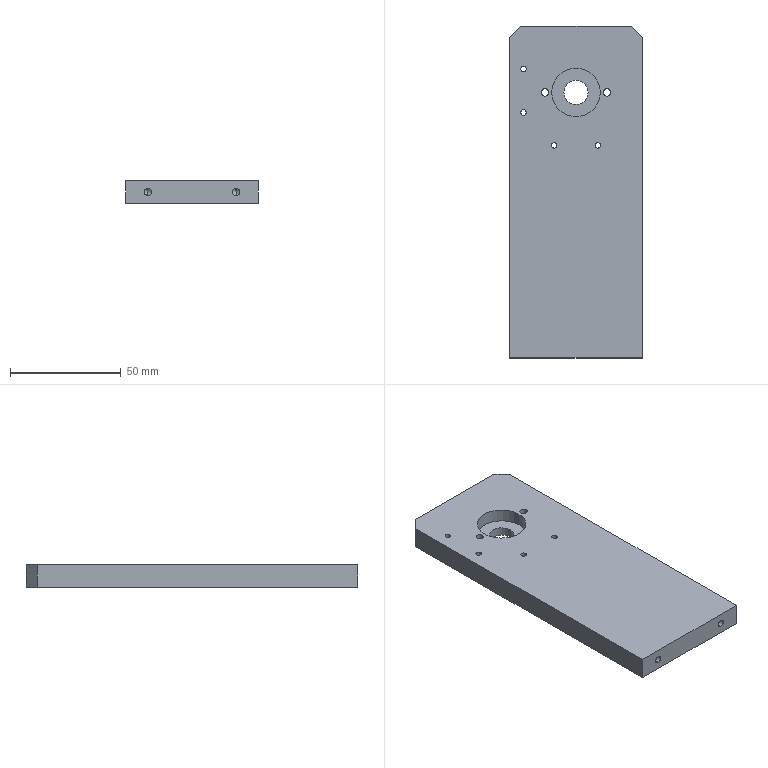Part | SolidWorks | features HoleWzd 3, ICE 2, Chamfer 1, Extrusion 1 | 1 solid | 33 faces | box 60 x 150 x 10 mm | volume 86519 mm3 | cylinder 20 | plane 9 | cone 4 | commonest cylinder face diameters 2.5 x8 3.3 x8 11 x2 22 x2
STEP:
#1=CARTESIAN_POINT('',(11.1,21.1,10.));
#2=VERTEX_POINT('',#1);
#3=CARTESIAN_POINT('',(8.6,21.1,10.));
#4=VERTEX_POINT('',#3);
#5=CARTESIAN_POINT('',(9.85,21.1,10.));
#6=DIRECTION('',(0.,0.,-1.));
#7=DIRECTION('',(-1.,0.,0.));
#8=AXIS2_PLACEMENT_3D('',#5,#6,#7);
#9=CIRCLE('',#8,1.25);
#10=EDGE_CURVE('',#2,#4,#9,.T.);
#11=ORIENTED_EDGE('',*,*,#10,.F.);
#12=CARTESIAN_POINT('',(11.1,21.1,0.));
#13=VERTEX_POINT('',#12);
#14=CARTESIAN_POINT('',(11.1,21.1,0.));
#15=DIRECTION('',(0.,0.,-1.));
#16=VECTOR('',#15,1000.);
#17=LINE('',#14,#16);
#18=EDGE_CURVE('',#2,#13,#17,.T.);
#19=ORIENTED_EDGE('',*,*,#18,.T.);
#20=CARTESIAN_POINT('',(8.6,21.1,0.));
#21=VERTEX_POINT('',#20);
#22=CARTESIAN_POINT('',(9.85,21.1,0.));
#23=DIRECTION('',(0.,0.,-1.));
#24=DIRECTION('',(-1.,0.,0.));
#25=AXIS2_PLACEMENT_3D('',#22,#23,#24);
#26=CIRCLE('',#25,1.25);
#27=EDGE_CURVE('',#13,#21,#26,.T.);
#28=ORIENTED_EDGE('',*,*,#27,.T.);
#29=CARTESIAN_POINT('',(8.6,21.1,0.));
#30=DIRECTION('',(0.,0.,-1.));
#31=VECTOR('',#30,1000.);
#32=LINE('',#29,#31);
#33=EDGE_CURVE('',#4,#21,#32,.T.);
#34=ORIENTED_EDGE('',*,*,#33,.F.);
#35=EDGE_LOOP('',(#11,#19,#28,#34));
#36=FACE_OUTER_BOUND('',#35,.T.);
#37=CARTESIAN_POINT('',(9.85,21.1,0.));
#38=DIRECTION('',(0.,0.,-1.));
#39=DIRECTION('',(-1.,0.,0.));
#40=AXIS2_PLACEMENT_3D('',#37,#38,#39);
#41=CYLINDRICAL_SURFACE('',#40,1.25);
#42=ADVANCED_FACE('',(#36),#41,.F.);
#43=CARTESIAN_POINT('',(-8.6,21.1,10.));
#44=VERTEX_POINT('',#43);
#45=CARTESIAN_POINT('',(-11.1,21.1,10.));
#46=VERTEX_POINT('',#45);
#47=CARTESIAN_POINT('',(-9.85,21.1,10.));
#48=DIRECTION('',(0.,0.,-1.));
#49=DIRECTION('',(-1.,0.,0.));
#50=AXIS2_PLACEMENT_3D('',#47,#48,#49);
#51=CIRCLE('',#50,1.25);
#52=EDGE_CURVE('',#44,#46,#51,.T.);
#53=ORIENTED_EDGE('',*,*,#52,.F.);
#54=CARTESIAN_POINT('',(-8.6,21.1,0.));
#55=VERTEX_POINT('',#54);
#56=CARTESIAN_POINT('',(-8.6,21.1,0.));
#57=DIRECTION('',(0.,0.,-1.));
#58=VECTOR('',#57,1000.);
#59=LINE('',#56,#58);
#60=EDGE_CURVE('',#44,#55,#59,.T.);
#61=ORIENTED_EDGE('',*,*,#60,.T.);
#62=CARTESIAN_POINT('',(-11.1,21.1,0.));
#63=VERTEX_POINT('',#62);
#64=CARTESIAN_POINT('',(-9.85,21.1,0.));
#65=DIRECTION('',(0.,0.,-1.));
#66=DIRECTION('',(-1.,0.,0.));
#67=AXIS2_PLACEMENT_3D('',#64,#65,#66);
#68=CIRCLE('',#67,1.25);
#69=EDGE_CURVE('',#55,#63,#68,.T.);
#70=ORIENTED_EDGE('',*,*,#69,.T.);
#71=CARTESIAN_POINT('',(-11.1,21.1,0.));
#72=DIRECTION('',(0.,0.,-1.));
#73=VECTOR('',#72,1000.);
#74=LINE('',#71,#73);
#75=EDGE_CURVE('',#46,#63,#74,.T.);
#76=ORIENTED_EDGE('',*,*,#75,.F.);
#77=EDGE_LOOP('',(#53,#61,#70,#76));
#78=FACE_OUTER_BOUND('',#77,.T.);
#79=CARTESIAN_POINT('',(-9.85,21.1,0.));
#80=DIRECTION('',(0.,0.,-1.));
#81=DIRECTION('',(-1.,0.,0.));
#82=AXIS2_PLACEMENT_3D('',#79,#80,#81);
#83=CYLINDRICAL_SURFACE('',#82,1.25);
#84=ADVANCED_FACE('',(#78),#83,.F.);
#85=CARTESIAN_POINT('',(-22.45,35.95,10.));
#86=VERTEX_POINT('',#85);
#87=CARTESIAN_POINT('',(-24.95,35.95,10.));
#88=VERTEX_POINT('',#87);
#89=CARTESIAN_POINT('',(-23.7,35.95,10.));
#90=DIRECTION('',(0.,0.,-1.));
#91=DIRECTION('',(-1.,0.,0.));
#92=AXIS2_PLACEMENT_3D('',#89,#90,#91);
#93=CIRCLE('',#92,1.25);
#94=EDGE_CURVE('',#86,#88,#93,.T.);
#95=ORIENTED_EDGE('',*,*,#94,.F.);
#96=CARTESIAN_POINT('',(-22.45,35.95,0.));
#97=VERTEX_POINT('',#96);
#98=CARTESIAN_POINT('',(-22.45,35.95,0.));
#99=DIRECTION('',(0.,0.,-1.));
#100=VECTOR('',#99,1000.);
#101=LINE('',#98,#100);
#102=EDGE_CURVE('',#86,#97,#101,.T.);
#103=ORIENTED_EDGE('',*,*,#102,.T.);
#104=CARTESIAN_POINT('',(-24.95,35.95,0.));
#105=VERTEX_POINT('',#104);
#106=CARTESIAN_POINT('',(-23.7,35.95,0.));
#107=DIRECTION('',(0.,0.,-1.));
#108=DIRECTION('',(-1.,0.,0.));
#109=AXIS2_PLACEMENT_3D('',#106,#107,#108);
#110=CIRCLE('',#109,1.25);
#111=EDGE_CURVE('',#97,#105,#110,.T.);
#112=ORIENTED_EDGE('',*,*,#111,.T.);
#113=CARTESIAN_POINT('',(-24.95,35.95,0.));
#114=DIRECTION('',(0.,0.,-1.));
#115=VECTOR('',#114,1000.);
#116=LINE('',#113,#115);
#117=EDGE_CURVE('',#88,#105,#116,.T.);
#118=ORIENTED_EDGE('',*,*,#117,.F.);
#119=EDGE_LOOP('',(#95,#103,#112,#118));
#120=FACE_OUTER_BOUND('',#119,.T.);
#121=CARTESIAN_POINT('',(-23.7,35.95,0.));
#122=DIRECTION('',(0.,0.,-1.));
#123=DIRECTION('',(-1.,0.,0.));
#124=AXIS2_PLACEMENT_3D('',#121,#122,#123);
#125=CYLINDRICAL_SURFACE('',#124,1.25);
#126=ADVANCED_FACE('',(#120),#125,.F.);
#127=CARTESIAN_POINT('',(-22.45,55.65,10.));
#128=VERTEX_POINT('',#127);
#129=CARTESIAN_POINT('',(-24.95,55.65,10.));
#130=VERTEX_POINT('',#129);
#131=CARTESIAN_POINT('',(-23.7,55.65,10.));
#132=DIRECTION('',(0.,0.,-1.));
#133=DIRECTION('',(-1.,0.,0.));
#134=AXIS2_PLACEMENT_3D('',#131,#132,#133);
#135=CIRCLE('',#134,1.25);
#136=EDGE_CURVE('',#128,#130,#135,.T.);
#137=ORIENTED_EDGE('',*,*,#136,.F.);
#138=CARTESIAN_POINT('',(-22.45,55.65,0.));
#139=VERTEX_POINT('',#138);
#140=CARTESIAN_POINT('',(-22.45,55.65,0.));
#141=DIRECTION('',(0.,0.,-1.));
#142=VECTOR('',#141,1000.);
#143=LINE('',#140,#142);
#144=EDGE_CURVE('',#128,#139,#143,.T.);
#145=ORIENTED_EDGE('',*,*,#144,.T.);
#146=CARTESIAN_POINT('',(-24.95,55.65,0.));
#147=VERTEX_POINT('',#146);
#148=CARTESIAN_POINT('',(-23.7,55.65,0.));
#149=DIRECTION('',(0.,0.,-1.));
#150=DIRECTION('',(-1.,0.,0.));
#151=AXIS2_PLACEMENT_3D('',#148,#149,#150);
#152=CIRCLE('',#151,1.25);
#153=EDGE_CURVE('',#139,#147,#152,.T.);
#154=ORIENTED_EDGE('',*,*,#153,.T.);
#155=CARTESIAN_POINT('',(-24.95,55.65,0.));
#156=DIRECTION('',(0.,0.,-1.));
#157=VECTOR('',#156,1000.);
#158=LINE('',#155,#157);
#159=EDGE_CURVE('',#130,#147,#158,.T.);
#160=ORIENTED_EDGE('',*,*,#159,.F.);
#161=EDGE_LOOP('',(#137,#145,#154,#160));
#162=FACE_OUTER_BOUND('',#161,.T.);
#163=CARTESIAN_POINT('',(-23.7,55.65,0.));
#164=DIRECTION('',(0.,0.,-1.));
#165=DIRECTION('',(-1.,0.,0.));
#166=AXIS2_PLACEMENT_3D('',#163,#164,#165);
#167=CYLINDRICAL_SURFACE('',#166,1.25);
#168=ADVANCED_FACE('',(#162),#167,.F.);
#169=CARTESIAN_POINT('',(20.,-63.5,6.65));
#170=VERTEX_POINT('',#169);
#171=CARTESIAN_POINT('',(20.,-63.5,3.35));
#172=VERTEX_POINT('',#171);
#173=CARTESIAN_POINT('',(20.,-63.5,5.));
#174=DIRECTION('',(0.,-1.,0.));
#175=DIRECTION('',(0.,0.,-1.));
#176=AXIS2_PLACEMENT_3D('',#173,#174,#175);
#177=CIRCLE('',#176,1.65);
#178=EDGE_CURVE('',#170,#172,#177,.T.);
#179=ORIENTED_EDGE('',*,*,#178,.F.);
#180=CARTESIAN_POINT('',(20.,-75.,6.65));
#181=VERTEX_POINT('',#180);
#182=CARTESIAN_POINT('',(20.,-75.,6.65));
#183=DIRECTION('',(0.,-1.,0.));
#184=VECTOR('',#183,1000.);
#185=LINE('',#182,#184);
#186=EDGE_CURVE('',#170,#181,#185,.T.);
#187=ORIENTED_EDGE('',*,*,#186,.T.);
#188=CARTESIAN_POINT('',(20.,-75.,3.35));
#189=VERTEX_POINT('',#188);
#190=CARTESIAN_POINT('',(20.,-75.,5.));
#191=DIRECTION('',(0.,-1.,0.));
#192=DIRECTION('',(0.,0.,-1.));
#193=AXIS2_PLACEMENT_3D('',#190,#191,#192);
#194=CIRCLE('',#193,1.65);
#195=EDGE_CURVE('',#181,#189,#194,.T.);
#196=ORIENTED_EDGE('',*,*,#195,.T.);
#197=CARTESIAN_POINT('',(20.,-75.,3.35));
#198=DIRECTION('',(0.,-1.,0.));
#199=VECTOR('',#198,1000.);
#200=LINE('',#197,#199);
#201=EDGE_CURVE('',#172,#189,#200,.T.);
#202=ORIENTED_EDGE('',*,*,#201,.F.);
#203=EDGE_LOOP('',(#179,#187,#196,#202));
#204=FACE_OUTER_BOUND('',#203,.T.);
#205=CARTESIAN_POINT('',(20.,-75.,5.));
#206=DIRECTION('',(0.,-1.,0.));
#207=DIRECTION('',(0.,0.,-1.));
#208=AXIS2_PLACEMENT_3D('',#205,#206,#207);
#209=CYLINDRICAL_SURFACE('',#208,1.65);
#210=ADVANCED_FACE('',(#204),#209,.F.);
#211=CARTESIAN_POINT('',(20.,-62.509,5.));
#212=VERTEX_POINT('',#211);
#213=CARTESIAN_POINT('',(20.,-63.5,3.35));
#214=DIRECTION('',(0.,-0.515,-0.8572));
#215=VECTOR('',#214,1000.);
#216=LINE('',#213,#215);
#217=EDGE_CURVE('',#212,#172,#216,.T.);
#218=ORIENTED_EDGE('',*,*,#217,.F.);
#219=CARTESIAN_POINT('',(20.,-63.5,6.65));
#220=DIRECTION('',(0.,-0.515,0.8572));
#221=VECTOR('',#220,1000.);
#222=LINE('',#219,#221);
#223=EDGE_CURVE('',#212,#170,#222,.T.);
#224=ORIENTED_EDGE('',*,*,#223,.T.);
#225=ORIENTED_EDGE('',*,*,#178,.T.);
#226=EDGE_LOOP('',(#218,#224,#225));
#227=FACE_OUTER_BOUND('',#226,.T.);
#228=CARTESIAN_POINT('',(20.,-63.5,5.));
#229=DIRECTION('',(0.,-1.,0.));
#230=DIRECTION('',(0.,0.,-1.));
#231=AXIS2_PLACEMENT_3D('',#228,#229,#230);
#232=CONICAL_SURFACE('',#231,1.65,1.03);
#233=ADVANCED_FACE('',(#227),#232,.F.);
#234=CARTESIAN_POINT('',(-20.,-63.5,6.65));
#235=VERTEX_POINT('',#234);
#236=CARTESIAN_POINT('',(-20.,-63.5,3.35));
#237=VERTEX_POINT('',#236);
#238=CARTESIAN_POINT('',(-20.,-63.5,5.));
#239=DIRECTION('',(0.,-1.,0.));
#240=DIRECTION('',(0.,0.,-1.));
#241=AXIS2_PLACEMENT_3D('',#238,#239,#240);
#242=CIRCLE('',#241,1.65);
#243=EDGE_CURVE('',#235,#237,#242,.T.);
#244=ORIENTED_EDGE('',*,*,#243,.F.);
#245=CARTESIAN_POINT('',(-20.,-75.,6.65));
#246=VERTEX_POINT('',#245);
#247=CARTESIAN_POINT('',(-20.,-75.,6.65));
#248=DIRECTION('',(0.,-1.,0.));
#249=VECTOR('',#248,1000.);
#250=LINE('',#247,#249);
#251=EDGE_CURVE('',#235,#246,#250,.T.);
#252=ORIENTED_EDGE('',*,*,#251,.T.);
#253=CARTESIAN_POINT('',(-20.,-75.,3.35));
#254=VERTEX_POINT('',#253);
#255=CARTESIAN_POINT('',(-20.,-75.,5.));
#256=DIRECTION('',(0.,-1.,0.));
#257=DIRECTION('',(0.,0.,-1.));
#258=AXIS2_PLACEMENT_3D('',#255,#256,#257);
#259=CIRCLE('',#258,1.65);
#260=EDGE_CURVE('',#246,#254,#259,.T.);
#261=ORIENTED_EDGE('',*,*,#260,.T.);
#262=CARTESIAN_POINT('',(-20.,-75.,3.35));
#263=DIRECTION('',(0.,-1.,0.));
#264=VECTOR('',#263,1000.);
#265=LINE('',#262,#264);
#266=EDGE_CURVE('',#237,#254,#265,.T.);
#267=ORIENTED_EDGE('',*,*,#266,.F.);
#268=EDGE_LOOP('',(#244,#252,#261,#267));
#269=FACE_OUTER_BOUND('',#268,.T.);
#270=CARTESIAN_POINT('',(-20.,-75.,5.));
#271=DIRECTION('',(0.,-1.,0.));
#272=DIRECTION('',(0.,0.,-1.));
#273=AXIS2_PLACEMENT_3D('',#270,#271,#272);
#274=CYLINDRICAL_SURFACE('',#273,1.65);
#275=ADVANCED_FACE('',(#269),#274,.F.);
#276=CARTESIAN_POINT('',(-20.,-62.509,5.));
#277=VERTEX_POINT('',#276);
#278=CARTESIAN_POINT('',(-20.,-63.5,3.35));
#279=DIRECTION('',(0.,-0.515,-0.8572));
#280=VECTOR('',#279,1000.);
#281=LINE('',#278,#280);
#282=EDGE_CURVE('',#277,#237,#281,.T.);
#283=ORIENTED_EDGE('',*,*,#282,.F.);
#284=CARTESIAN_POINT('',(-20.,-63.5,6.65));
#285=DIRECTION('',(0.,-0.515,0.8572));
#286=VECTOR('',#285,1000.);
#287=LINE('',#284,#286);
#288=EDGE_CURVE('',#277,#235,#287,.T.);
#289=ORIENTED_EDGE('',*,*,#288,.T.);
#290=ORIENTED_EDGE('',*,*,#243,.T.);
#291=EDGE_LOOP('',(#283,#289,#290));
#292=FACE_OUTER_BOUND('',#291,.T.);
#293=CARTESIAN_POINT('',(-20.,-63.5,5.));
#294=DIRECTION('',(0.,-1.,0.));
#295=DIRECTION('',(0.,0.,-1.));
#296=AXIS2_PLACEMENT_3D('',#293,#294,#295);
#297=CONICAL_SURFACE('',#296,1.65,1.03);
#298=ADVANCED_FACE('',(#292),#297,.F.);
#299=CARTESIAN_POINT('',(-15.65,45.,0.));
#300=VERTEX_POINT('',#299);
#301=CARTESIAN_POINT('',(-12.35,45.,0.));
#302=VERTEX_POINT('',#301);
#303=CARTESIAN_POINT('',(-14.,45.,0.));
#304=DIRECTION('',(0.,0.,1.));
#305=DIRECTION('',(1.,0.,0.));
#306=AXIS2_PLACEMENT_3D('',#303,#304,#305);
#307=CIRCLE('',#306,1.65);
#308=EDGE_CURVE('',#300,#302,#307,.T.);
#309=ORIENTED_EDGE('',*,*,#308,.F.);
#310=CARTESIAN_POINT('',(-15.65,45.,10.));
#311=VERTEX_POINT('',#310);
#312=CARTESIAN_POINT('',(-15.65,45.,10.));
#313=DIRECTION('',(0.,0.,1.));
#314=VECTOR('',#313,1000.);
#315=LINE('',#312,#314);
#316=EDGE_CURVE('',#300,#311,#315,.T.);
#317=ORIENTED_EDGE('',*,*,#316,.T.);
#318=CARTESIAN_POINT('',(-12.35,45.,10.));
#319=VERTEX_POINT('',#318);
#320=CARTESIAN_POINT('',(-14.,45.,10.));
#321=DIRECTION('',(0.,0.,1.));
#322=DIRECTION('',(1.,0.,0.));
#323=AXIS2_PLACEMENT_3D('',#320,#321,#322);
#324=CIRCLE('',#323,1.65);
#325=EDGE_CURVE('',#311,#319,#324,.T.);
#326=ORIENTED_EDGE('',*,*,#325,.T.);
#327=CARTESIAN_POINT('',(-12.35,45.,10.));
#328=DIRECTION('',(0.,0.,1.));
#329=VECTOR('',#328,1000.);
#330=LINE('',#327,#329);
#331=EDGE_CURVE('',#302,#319,#330,.T.);
#332=ORIENTED_EDGE('',*,*,#331,.F.);
#333=EDGE_LOOP('',(#309,#317,#326,#332));
#334=FACE_OUTER_BOUND('',#333,.T.);
#335=CARTESIAN_POINT('',(-14.,45.,10.));
#336=DIRECTION('',(0.,0.,1.));
#337=DIRECTION('',(1.,0.,0.));
#338=AXIS2_PLACEMENT_3D('',#335,#336,#337);
#339=CYLINDRICAL_SURFACE('',#338,1.65);
#340=ADVANCED_FACE('',(#334),#339,.F.);
#341=CARTESIAN_POINT('',(12.35,45.,0.));
#342=VERTEX_POINT('',#341);
#343=CARTESIAN_POINT('',(15.65,45.,0.));
#344=VERTEX_POINT('',#343);
#345=CARTESIAN_POINT('',(14.,45.,0.));
#346=DIRECTION('',(0.,0.,1.));
#347=DIRECTION('',(1.,0.,0.));
#348=AXIS2_PLACEMENT_3D('',#345,#346,#347);
#349=CIRCLE('',#348,1.65);
#350=EDGE_CURVE('',#342,#344,#349,.T.);
#351=ORIENTED_EDGE('',*,*,#350,.F.);
#352=CARTESIAN_POINT('',(12.35,45.,10.));
#353=VERTEX_POINT('',#352);
#354=CARTESIAN_POINT('',(12.35,45.,10.));
#355=DIRECTION('',(0.,0.,1.));
#356=VECTOR('',#355,1000.);
#357=LINE('',#354,#356);
#358=EDGE_CURVE('',#342,#353,#357,.T.);
#359=ORIENTED_EDGE('',*,*,#358,.T.);
#360=CARTESIAN_POINT('',(15.65,45.,10.));
#361=VERTEX_POINT('',#360);
#362=CARTESIAN_POINT('',(14.,45.,10.));
#363=DIRECTION('',(0.,0.,1.));
#364=DIRECTION('',(1.,0.,0.));
#365=AXIS2_PLACEMENT_3D('',#362,#363,#364);
#366=CIRCLE('',#365,1.65);
#367=EDGE_CURVE('',#353,#361,#366,.T.);
#368=ORIENTED_EDGE('',*,*,#367,.T.);
#369=CARTESIAN_POINT('',(15.65,45.,10.));
#370=DIRECTION('',(0.,0.,1.));
#371=VECTOR('',#370,1000.);
#372=LINE('',#369,#371);
#373=EDGE_CURVE('',#344,#361,#372,.T.);
#374=ORIENTED_EDGE('',*,*,#373,.F.);
#375=EDGE_LOOP('',(#351,#359,#368,#374));
#376=FACE_OUTER_BOUND('',#375,.T.);
#377=CARTESIAN_POINT('',(14.,45.,10.));
#378=DIRECTION('',(0.,0.,1.));
#379=DIRECTION('',(1.,0.,0.));
#380=AXIS2_PLACEMENT_3D('',#377,#378,#379);
#381=CYLINDRICAL_SURFACE('',#380,1.65);
#382=ADVANCED_FACE('',(#376),#381,.F.);
#383=CARTESIAN_POINT('',(-5.5,45.,0.));
#384=VERTEX_POINT('',#383);
#385=CARTESIAN_POINT('',(5.5,45.,0.));
#386=VERTEX_POINT('',#385);
#387=CARTESIAN_POINT('',(0.,45.,0.));
#388=DIRECTION('',(0.,0.,1.));
#389=DIRECTION('',(1.,0.,0.));
#390=AXIS2_PLACEMENT_3D('',#387,#388,#389);
#391=CIRCLE('',#390,5.5);
#392=EDGE_CURVE('',#384,#386,#391,.T.);
#393=ORIENTED_EDGE('',*,*,#392,.F.);
#394=CARTESIAN_POINT('',(-5.5,45.,4.));
#395=VERTEX_POINT('',#394);
#396=CARTESIAN_POINT('',(-5.5,45.,0.));
#397=DIRECTION('',(0.,0.,1.));
#398=VECTOR('',#397,1000.);
#399=LINE('',#396,#398);
#400=EDGE_CURVE('',#384,#395,#399,.T.);
#401=ORIENTED_EDGE('',*,*,#400,.T.);
#402=CARTESIAN_POINT('',(5.5,45.,4.));
#403=VERTEX_POINT('',#402);
#404=CARTESIAN_POINT('',(0.,45.,4.));
#405=DIRECTION('',(0.,0.,1.));
#406=DIRECTION('',(1.,0.,0.));
#407=AXIS2_PLACEMENT_3D('',#404,#405,#406);
#408=CIRCLE('',#407,5.5);
#409=EDGE_CURVE('',#395,#403,#408,.T.);
#410=ORIENTED_EDGE('',*,*,#409,.T.);
#411=CARTESIAN_POINT('',(5.5,45.,0.));
#412=DIRECTION('',(0.,0.,1.));
#413=VECTOR('',#412,1000.);
#414=LINE('',#411,#413);
#415=EDGE_CURVE('',#386,#403,#414,.T.);
#416=ORIENTED_EDGE('',*,*,#415,.F.);
#417=EDGE_LOOP('',(#393,#401,#410,#416));
#418=FACE_OUTER_BOUND('',#417,.T.);
#419=CARTESIAN_POINT('',(0.,45.,0.));
#420=DIRECTION('',(0.,0.,1.));
#421=DIRECTION('',(1.,0.,0.));
#422=AXIS2_PLACEMENT_3D('',#419,#420,#421);
#423=CYLINDRICAL_SURFACE('',#422,5.5);
#424=ADVANCED_FACE('',(#418),#423,.F.);
#425=CARTESIAN_POINT('',(-11.,45.,4.));
#426=VERTEX_POINT('',#425);
#427=CARTESIAN_POINT('',(11.,45.,4.));
#428=VERTEX_POINT('',#427);
#429=CARTESIAN_POINT('',(0.,45.,4.));
#430=DIRECTION('',(0.,0.,1.));
#431=DIRECTION('',(1.,0.,0.));
#432=AXIS2_PLACEMENT_3D('',#429,#430,#431);
#433=CIRCLE('',#432,11.);
#434=EDGE_CURVE('',#426,#428,#433,.T.);
#435=ORIENTED_EDGE('',*,*,#434,.F.);
#436=CARTESIAN_POINT('',(-11.,45.,10.));
#437=VERTEX_POINT('',#436);
#438=CARTESIAN_POINT('',(-11.,45.,4.));
#439=DIRECTION('',(0.,0.,1.));
#440=VECTOR('',#439,1000.);
#441=LINE('',#438,#440);
#442=EDGE_CURVE('',#426,#437,#441,.T.);
#443=ORIENTED_EDGE('',*,*,#442,.T.);
#444=CARTESIAN_POINT('',(11.,45.,10.));
#445=VERTEX_POINT('',#444);
#446=CARTESIAN_POINT('',(0.,45.,10.));
#447=DIRECTION('',(0.,0.,1.));
#448=DIRECTION('',(1.,0.,0.));
#449=AXIS2_PLACEMENT_3D('',#446,#447,#448);
#450=CIRCLE('',#449,11.);
#451=EDGE_CURVE('',#437,#445,#450,.T.);
#452=ORIENTED_EDGE('',*,*,#451,.T.);
#453=CARTESIAN_POINT('',(11.,45.,4.));
#454=DIRECTION('',(0.,0.,1.));
#455=VECTOR('',#454,1000.);
#456=LINE('',#453,#455);
#457=EDGE_CURVE('',#428,#445,#456,.T.);
#458=ORIENTED_EDGE('',*,*,#457,.F.);
#459=EDGE_LOOP('',(#435,#443,#452,#458));
#460=FACE_OUTER_BOUND('',#459,.T.);
#461=CARTESIAN_POINT('',(0.,45.,4.));
#462=DIRECTION('',(0.,0.,1.));
#463=DIRECTION('',(1.,0.,0.));
#464=AXIS2_PLACEMENT_3D('',#461,#462,#463);
#465=CYLINDRICAL_SURFACE('',#464,11.);
#466=ADVANCED_FACE('',(#460),#465,.F.);
#467=CARTESIAN_POINT('',(30.,-75.,0.));
#468=VERTEX_POINT('',#467);
#469=CARTESIAN_POINT('',(30.,70.,0.));
#470=VERTEX_POINT('',#469);
#471=CARTESIAN_POINT('',(30.,75.,0.));
#472=DIRECTION('',(0.,1.,0.));
#473=VECTOR('',#472,1000.);
#474=LINE('',#471,#473);
#475=EDGE_CURVE('',#468,#470,#474,.T.);
#476=ORIENTED_EDGE('',*,*,#475,.T.);
#477=CARTESIAN_POINT('',(30.,70.,10.));
#478=VERTEX_POINT('',#477);
#479=CARTESIAN_POINT('',(30.,70.,10.));
#480=DIRECTION('',(0.,0.,1.));
#481=VECTOR('',#480,1000.);
#482=LINE('',#479,#481);
#483=EDGE_CURVE('',#470,#478,#482,.T.);
#484=ORIENTED_EDGE('',*,*,#483,.T.);
#485=CARTESIAN_POINT('',(30.,-75.,10.));
#486=VERTEX_POINT('',#485);
#487=CARTESIAN_POINT('',(30.,75.,10.));
#488=DIRECTION('',(0.,1.,0.));
#489=VECTOR('',#488,1000.);
#490=LINE('',#487,#489);
#491=EDGE_CURVE('',#486,#478,#490,.T.);
#492=ORIENTED_EDGE('',*,*,#491,.F.);
#493=CARTESIAN_POINT('',(30.,-75.,10.));
#494=DIRECTION('',(0.,0.,-1.));
#495=VECTOR('',#494,1000.);
#496=LINE('',#493,#495);
#497=EDGE_CURVE('',#486,#468,#496,.T.);
#498=ORIENTED_EDGE('',*,*,#497,.T.);
#499=EDGE_LOOP('',(#476,#484,#492,#498));
#500=FACE_OUTER_BOUND('',#499,.T.);
#501=CARTESIAN_POINT('',(30.,75.,10.));
#502=DIRECTION('',(-1.,0.,0.));
#503=DIRECTION('',(0.,-1.,0.));
#504=AXIS2_PLACEMENT_3D('',#501,#502,#503);
#505=PLANE('',#504);
#506=ADVANCED_FACE('',(#500),#505,.F.);
#507=CARTESIAN_POINT('',(25.,75.,10.));
#508=VERTEX_POINT('',#507);
#509=CARTESIAN_POINT('',(-25.,75.,10.));
#510=VERTEX_POINT('',#509);
#511=CARTESIAN_POINT('',(-30.,75.,10.));
#512=DIRECTION('',(-1.,0.,0.));
#513=VECTOR('',#512,1000.);
#514=LINE('',#511,#513);
#515=EDGE_CURVE('',#508,#510,#514,.T.);
#516=ORIENTED_EDGE('',*,*,#515,.F.);
#517=CARTESIAN_POINT('',(25.,75.,0.));
#518=VERTEX_POINT('',#517);
#519=CARTESIAN_POINT('',(25.,75.,10.));
#520=DIRECTION('',(0.,0.,-1.));
#521=VECTOR('',#520,1000.);
#522=LINE('',#519,#521);
#523=EDGE_CURVE('',#508,#518,#522,.T.);
#524=ORIENTED_EDGE('',*,*,#523,.T.);
#525=CARTESIAN_POINT('',(-25.,75.,0.));
#526=VERTEX_POINT('',#525);
#527=CARTESIAN_POINT('',(-30.,75.,0.));
#528=DIRECTION('',(-1.,0.,0.));
#529=VECTOR('',#528,1000.);
#530=LINE('',#527,#529);
#531=EDGE_CURVE('',#518,#526,#530,.T.);
#532=ORIENTED_EDGE('',*,*,#531,.T.);
#533=CARTESIAN_POINT('',(-25.,75.,10.));
#534=DIRECTION('',(0.,0.,1.));
#535=VECTOR('',#534,1000.);
#536=LINE('',#533,#535);
#537=EDGE_CURVE('',#526,#510,#536,.T.);
#538=ORIENTED_EDGE('',*,*,#537,.T.);
#539=EDGE_LOOP('',(#516,#524,#532,#538));
#540=FACE_OUTER_BOUND('',#539,.T.);
#541=CARTESIAN_POINT('',(-30.,75.,10.));
#542=DIRECTION('',(0.,-1.,0.));
#543=DIRECTION('',(0.,0.,-1.));
#544=AXIS2_PLACEMENT_3D('',#541,#542,#543);
#545=PLANE('',#544);
#546=ADVANCED_FACE('',(#540),#545,.F.);
#547=CARTESIAN_POINT('',(-30.,70.,10.));
#548=VERTEX_POINT('',#547);
#549=CARTESIAN_POINT('',(-30.,-75.,10.));
#550=VERTEX_POINT('',#549);
#551=CARTESIAN_POINT('',(-30.,75.,10.));
#552=DIRECTION('',(0.,-1.,0.));
#553=VECTOR('',#552,1000.);
#554=LINE('',#551,#553);
#555=EDGE_CURVE('',#548,#550,#554,.T.);
#556=ORIENTED_EDGE('',*,*,#555,.F.);
#557=CARTESIAN_POINT('',(-30.,70.,0.));
#558=VERTEX_POINT('',#557);
#559=CARTESIAN_POINT('',(-30.,70.,10.));
#560=DIRECTION('',(0.,0.,-1.));
#561=VECTOR('',#560,1000.);
#562=LINE('',#559,#561);
#563=EDGE_CURVE('',#548,#558,#562,.T.);
#564=ORIENTED_EDGE('',*,*,#563,.T.);
#565=CARTESIAN_POINT('',(-30.,-75.,0.));
#566=VERTEX_POINT('',#565);
#567=CARTESIAN_POINT('',(-30.,75.,0.));
#568=DIRECTION('',(0.,-1.,0.));
#569=VECTOR('',#568,1000.);
#570=LINE('',#567,#569);
#571=EDGE_CURVE('',#558,#566,#570,.T.);
#572=ORIENTED_EDGE('',*,*,#571,.T.);
#573=CARTESIAN_POINT('',(-30.,-75.,10.));
#574=DIRECTION('',(0.,0.,-1.));
#575=VECTOR('',#574,1000.);
#576=LINE('',#573,#575);
#577=EDGE_CURVE('',#550,#566,#576,.T.);
#578=ORIENTED_EDGE('',*,*,#577,.F.);
#579=EDGE_LOOP('',(#556,#564,#572,#578));
#580=FACE_OUTER_BOUND('',#579,.T.);
#581=CARTESIAN_POINT('',(-30.,75.,10.));
#582=DIRECTION('',(1.,0.,0.));
#583=DIRECTION('',(0.,1.,0.));
#584=AXIS2_PLACEMENT_3D('',#581,#582,#583);
#585=PLANE('',#584);
#586=ADVANCED_FACE('',(#580),#585,.F.);
#587=CARTESIAN_POINT('',(20.,-75.,5.));
#588=DIRECTION('',(0.,-1.,0.));
#589=DIRECTION('',(0.,0.,-1.));
#590=AXIS2_PLACEMENT_3D('',#587,#588,#589);
#591=CIRCLE('',#590,1.65);
#592=EDGE_CURVE('',#189,#181,#591,.T.);
#593=ORIENTED_EDGE('',*,*,#592,.F.);
#594=ORIENTED_EDGE('',*,*,#195,.F.);
#595=EDGE_LOOP('',(#593,#594));
#596=FACE_BOUND('',#595,.T.);
#597=CARTESIAN_POINT('',(-20.,-75.,5.));
#598=DIRECTION('',(0.,-1.,0.));
#599=DIRECTION('',(0.,0.,-1.));
#600=AXIS2_PLACEMENT_3D('',#597,#598,#599);
#601=CIRCLE('',#600,1.65);
#602=EDGE_CURVE('',#254,#246,#601,.T.);
#603=ORIENTED_EDGE('',*,*,#602,.F.);
#604=ORIENTED_EDGE('',*,*,#260,.F.);
#605=EDGE_LOOP('',(#603,#604));
#606=FACE_BOUND('',#605,.T.);
#607=CARTESIAN_POINT('',(-30.,-75.,0.));
#608=DIRECTION('',(1.,0.,0.));
#609=VECTOR('',#608,1000.);
#610=LINE('',#607,#609);
#611=EDGE_CURVE('',#566,#468,#610,.T.);
#612=ORIENTED_EDGE('',*,*,#611,.T.);
#613=ORIENTED_EDGE('',*,*,#497,.F.);
#614=CARTESIAN_POINT('',(-30.,-75.,10.));
#615=DIRECTION('',(1.,0.,0.));
#616=VECTOR('',#615,1000.);
#617=LINE('',#614,#616);
#618=EDGE_CURVE('',#550,#486,#617,.T.);
#619=ORIENTED_EDGE('',*,*,#618,.F.);
#620=ORIENTED_EDGE('',*,*,#577,.T.);
#621=EDGE_LOOP('',(#612,#613,#619,#620));
#622=FACE_OUTER_BOUND('',#621,.T.);
#623=CARTESIAN_POINT('',(-30.,-75.,10.));
#624=DIRECTION('',(0.,1.,0.));
#625=DIRECTION('',(0.,0.,1.));
#626=AXIS2_PLACEMENT_3D('',#623,#624,#625);
#627=PLANE('',#626);
#628=ADVANCED_FACE('',(#596,#606,#622),#627,.F.);
#629=CARTESIAN_POINT('',(9.85,21.1,10.));
#630=DIRECTION('',(0.,0.,-1.));
#631=DIRECTION('',(-1.,0.,0.));
#632=AXIS2_PLACEMENT_3D('',#629,#630,#631);
#633=CIRCLE('',#632,1.25);
#634=EDGE_CURVE('',#4,#2,#633,.T.);
#635=ORIENTED_EDGE('',*,*,#634,.T.);
#636=ORIENTED_EDGE('',*,*,#10,.T.);
#637=EDGE_LOOP('',(#635,#636));
#638=FACE_BOUND('',#637,.T.);
#639=CARTESIAN_POINT('',(-9.85,21.1,10.));
#640=DIRECTION('',(0.,0.,-1.));
#641=DIRECTION('',(-1.,0.,0.));
#642=AXIS2_PLACEMENT_3D('',#639,#640,#641);
#643=CIRCLE('',#642,1.25);
#644=EDGE_CURVE('',#46,#44,#643,.T.);
#645=ORIENTED_EDGE('',*,*,#644,.T.);
#646=ORIENTED_EDGE('',*,*,#52,.T.);
#647=EDGE_LOOP('',(#645,#646));
#648=FACE_BOUND('',#647,.T.);
#649=CARTESIAN_POINT('',(-23.7,35.95,10.));
#650=DIRECTION('',(0.,0.,-1.));
#651=DIRECTION('',(-1.,0.,0.));
#652=AXIS2_PLACEMENT_3D('',#649,#650,#651);
#653=CIRCLE('',#652,1.25);
#654=EDGE_CURVE('',#88,#86,#653,.T.);
#655=ORIENTED_EDGE('',*,*,#654,.T.);
#656=ORIENTED_EDGE('',*,*,#94,.T.);
#657=EDGE_LOOP('',(#655,#656));
#658=FACE_BOUND('',#657,.T.);
#659=CARTESIAN_POINT('',(-23.7,55.65,10.));
#660=DIRECTION('',(0.,0.,-1.));
#661=DIRECTION('',(-1.,0.,0.));
#662=AXIS2_PLACEMENT_3D('',#659,#660,#661);
#663=CIRCLE('',#662,1.25);
#664=EDGE_CURVE('',#130,#128,#663,.T.);
#665=ORIENTED_EDGE('',*,*,#664,.T.);
#666=ORIENTED_EDGE('',*,*,#136,.T.);
#667=EDGE_LOOP('',(#665,#666));
#668=FACE_BOUND('',#667,.T.);
#669=CARTESIAN_POINT('',(-14.,45.,10.));
#670=DIRECTION('',(0.,0.,1.));
#671=DIRECTION('',(1.,0.,0.));
#672=AXIS2_PLACEMENT_3D('',#669,#670,#671);
#673=CIRCLE('',#672,1.65);
#674=EDGE_CURVE('',#319,#311,#673,.T.);
#675=ORIENTED_EDGE('',*,*,#674,.F.);
#676=ORIENTED_EDGE('',*,*,#325,.F.);
#677=EDGE_LOOP('',(#675,#676));
#678=FACE_BOUND('',#677,.T.);
#679=CARTESIAN_POINT('',(14.,45.,10.));
#680=DIRECTION('',(0.,0.,1.));
#681=DIRECTION('',(1.,0.,0.));
#682=AXIS2_PLACEMENT_3D('',#679,#680,#681);
#683=CIRCLE('',#682,1.65);
#684=EDGE_CURVE('',#361,#353,#683,.T.);
#685=ORIENTED_EDGE('',*,*,#684,.F.);
#686=ORIENTED_EDGE('',*,*,#367,.F.);
#687=EDGE_LOOP('',(#685,#686));
#688=FACE_BOUND('',#687,.T.);
#689=CARTESIAN_POINT('',(0.,45.,10.));
#690=DIRECTION('',(0.,0.,1.));
#691=DIRECTION('',(1.,0.,0.));
#692=AXIS2_PLACEMENT_3D('',#689,#690,#691);
#693=CIRCLE('',#692,11.);
#694=EDGE_CURVE('',#445,#437,#693,.T.);
#695=ORIENTED_EDGE('',*,*,#694,.F.);
#696=ORIENTED_EDGE('',*,*,#451,.F.);
#697=EDGE_LOOP('',(#695,#696));
#698=FACE_BOUND('',#697,.T.);
#699=ORIENTED_EDGE('',*,*,#491,.T.);
#700=CARTESIAN_POINT('',(50.,50.,10.));
#701=DIRECTION('',(-0.7071,0.7071,0.));
#702=VECTOR('',#701,1000.);
#703=LINE('',#700,#702);
#704=EDGE_CURVE('',#478,#508,#703,.T.);
#705=ORIENTED_EDGE('',*,*,#704,.T.);
#706=ORIENTED_EDGE('',*,*,#515,.T.);
#707=CARTESIAN_POINT('',(-50.,50.,10.));
#708=DIRECTION('',(-0.7071,-0.7071,0.));
#709=VECTOR('',#708,1000.);
#710=LINE('',#707,#709);
#711=EDGE_CURVE('',#510,#548,#710,.T.);
#712=ORIENTED_EDGE('',*,*,#711,.T.);
#713=ORIENTED_EDGE('',*,*,#555,.T.);
#714=ORIENTED_EDGE('',*,*,#618,.T.);
#715=EDGE_LOOP('',(#699,#705,#706,#712,#713,#714));
#716=FACE_OUTER_BOUND('',#715,.T.);
#717=CARTESIAN_POINT('',(0.,0.,10.));
#718=DIRECTION('',(0.,0.,1.));
#719=DIRECTION('',(1.,0.,0.));
#720=AXIS2_PLACEMENT_3D('',#717,#718,#719);
#721=PLANE('',#720);
#722=ADVANCED_FACE('',(#638,#648,#658,#668,#678,#688,#698,#716),#721,.T.);
#723=CARTESIAN_POINT('',(9.85,21.1,0.));
#724=DIRECTION('',(0.,0.,-1.));
#725=DIRECTION('',(-1.,0.,0.));
#726=AXIS2_PLACEMENT_3D('',#723,#724,#725);
#727=CIRCLE('',#726,1.25);
#728=EDGE_CURVE('',#21,#13,#727,.T.);
#729=ORIENTED_EDGE('',*,*,#728,.F.);
#730=ORIENTED_EDGE('',*,*,#27,.F.);
#731=EDGE_LOOP('',(#729,#730));
#732=FACE_BOUND('',#731,.T.);
#733=CARTESIAN_POINT('',(-9.85,21.1,0.));
#734=DIRECTION('',(0.,0.,-1.));
#735=DIRECTION('',(-1.,0.,0.));
#736=AXIS2_PLACEMENT_3D('',#733,#734,#735);
#737=CIRCLE('',#736,1.25);
#738=EDGE_CURVE('',#63,#55,#737,.T.);
#739=ORIENTED_EDGE('',*,*,#738,.F.);
#740=ORIENTED_EDGE('',*,*,#69,.F.);
#741=EDGE_LOOP('',(#739,#740));
#742=FACE_BOUND('',#741,.T.);
#743=CARTESIAN_POINT('',(-23.7,35.95,0.));
#744=DIRECTION('',(0.,0.,-1.));
#745=DIRECTION('',(-1.,0.,0.));
#746=AXIS2_PLACEMENT_3D('',#743,#744,#745);
#747=CIRCLE('',#746,1.25);
#748=EDGE_CURVE('',#105,#97,#747,.T.);
#749=ORIENTED_EDGE('',*,*,#748,.F.);
#750=ORIENTED_EDGE('',*,*,#111,.F.);
#751=EDGE_LOOP('',(#749,#750));
#752=FACE_BOUND('',#751,.T.);
#753=CARTESIAN_POINT('',(-23.7,55.65,0.));
#754=DIRECTION('',(0.,0.,-1.));
#755=DIRECTION('',(-1.,0.,0.));
#756=AXIS2_PLACEMENT_3D('',#753,#754,#755);
#757=CIRCLE('',#756,1.25);
#758=EDGE_CURVE('',#147,#139,#757,.T.);
#759=ORIENTED_EDGE('',*,*,#758,.F.);
#760=ORIENTED_EDGE('',*,*,#153,.F.);
#761=EDGE_LOOP('',(#759,#760));
#762=FACE_BOUND('',#761,.T.);
#763=CARTESIAN_POINT('',(-14.,45.,0.));
#764=DIRECTION('',(0.,0.,1.));
#765=DIRECTION('',(1.,0.,0.));
#766=AXIS2_PLACEMENT_3D('',#763,#764,#765);
#767=CIRCLE('',#766,1.65);
#768=EDGE_CURVE('',#302,#300,#767,.T.);
#769=ORIENTED_EDGE('',*,*,#768,.T.);
#770=ORIENTED_EDGE('',*,*,#308,.T.);
#771=EDGE_LOOP('',(#769,#770));
#772=FACE_BOUND('',#771,.T.);
#773=CARTESIAN_POINT('',(14.,45.,0.));
#774=DIRECTION('',(0.,0.,1.));
#775=DIRECTION('',(1.,0.,0.));
#776=AXIS2_PLACEMENT_3D('',#773,#774,#775);
#777=CIRCLE('',#776,1.65);
#778=EDGE_CURVE('',#344,#342,#777,.T.);
#779=ORIENTED_EDGE('',*,*,#778,.T.);
#780=ORIENTED_EDGE('',*,*,#350,.T.);
#781=EDGE_LOOP('',(#779,#780));
#782=FACE_BOUND('',#781,.T.);
#783=CARTESIAN_POINT('',(0.,45.,0.));
#784=DIRECTION('',(0.,0.,1.));
#785=DIRECTION('',(1.,0.,0.));
#786=AXIS2_PLACEMENT_3D('',#783,#784,#785);
#787=CIRCLE('',#786,5.5);
#788=EDGE_CURVE('',#386,#384,#787,.T.);
#789=ORIENTED_EDGE('',*,*,#788,.T.);
#790=ORIENTED_EDGE('',*,*,#392,.T.);
#791=EDGE_LOOP('',(#789,#790));
#792=FACE_BOUND('',#791,.T.);
#793=ORIENTED_EDGE('',*,*,#531,.F.);
#794=CARTESIAN_POINT('',(25.,75.,0.));
#795=DIRECTION('',(0.7071,-0.7071,0.));
#796=VECTOR('',#795,1000.);
#797=LINE('',#794,#796);
#798=EDGE_CURVE('',#518,#470,#797,.T.);
#799=ORIENTED_EDGE('',*,*,#798,.T.);
#800=ORIENTED_EDGE('',*,*,#475,.F.);
#801=ORIENTED_EDGE('',*,*,#611,.F.);
#802=ORIENTED_EDGE('',*,*,#571,.F.);
#803=CARTESIAN_POINT('',(-30.,70.,0.));
#804=DIRECTION('',(0.7071,0.7071,0.));
#805=VECTOR('',#804,1000.);
#806=LINE('',#803,#805);
#807=EDGE_CURVE('',#558,#526,#806,.T.);
#808=ORIENTED_EDGE('',*,*,#807,.T.);
#809=EDGE_LOOP('',(#793,#799,#800,#801,#802,#808));
#810=FACE_OUTER_BOUND('',#809,.T.);
#811=CARTESIAN_POINT('',(0.,0.,0.));
#812=DIRECTION('',(0.,0.,1.));
#813=DIRECTION('',(1.,0.,0.));
#814=AXIS2_PLACEMENT_3D('',#811,#812,#813);
#815=PLANE('',#814);
#816=ADVANCED_FACE('',(#732,#742,#752,#762,#772,#782,#792,#810),#815,.F.);
#817=ORIENTED_EDGE('',*,*,#704,.F.);
#818=ORIENTED_EDGE('',*,*,#483,.F.);
#819=ORIENTED_EDGE('',*,*,#798,.F.);
#820=ORIENTED_EDGE('',*,*,#523,.F.);
#821=EDGE_LOOP('',(#817,#818,#819,#820));
#822=FACE_OUTER_BOUND('',#821,.T.);
#823=CARTESIAN_POINT('',(25.,75.,10.));
#824=DIRECTION('',(-0.7071,-0.7071,0.));
#825=DIRECTION('',(0.,0.,-1.));
#826=AXIS2_PLACEMENT_3D('',#823,#824,#825);
#827=PLANE('',#826);
#828=ADVANCED_FACE('',(#822),#827,.F.);
#829=ORIENTED_EDGE('',*,*,#711,.F.);
#830=ORIENTED_EDGE('',*,*,#537,.F.);
#831=ORIENTED_EDGE('',*,*,#807,.F.);
#832=ORIENTED_EDGE('',*,*,#563,.F.);
#833=EDGE_LOOP('',(#829,#830,#831,#832));
#834=FACE_OUTER_BOUND('',#833,.T.);
#835=CARTESIAN_POINT('',(-30.,70.,10.));
#836=DIRECTION('',(0.7071,-0.7071,0.));
#837=DIRECTION('',(0.,0.,-1.));
#838=AXIS2_PLACEMENT_3D('',#835,#836,#837);
#839=PLANE('',#838);
#840=ADVANCED_FACE('',(#834),#839,.F.);
#841=ORIENTED_EDGE('',*,*,#442,.F.);
#842=CARTESIAN_POINT('',(0.,45.,4.));
#843=DIRECTION('',(0.,0.,1.));
#844=DIRECTION('',(1.,0.,0.));
#845=AXIS2_PLACEMENT_3D('',#842,#843,#844);
#846=CIRCLE('',#845,11.);
#847=EDGE_CURVE('',#428,#426,#846,.T.);
#848=ORIENTED_EDGE('',*,*,#847,.F.);
#849=ORIENTED_EDGE('',*,*,#457,.T.);
#850=ORIENTED_EDGE('',*,*,#694,.T.);
#851=EDGE_LOOP('',(#841,#848,#849,#850));
#852=FACE_OUTER_BOUND('',#851,.T.);
#853=CARTESIAN_POINT('',(0.,45.,4.));
#854=DIRECTION('',(0.,0.,1.));
#855=DIRECTION('',(1.,0.,0.));
#856=AXIS2_PLACEMENT_3D('',#853,#854,#855);
#857=CYLINDRICAL_SURFACE('',#856,11.);
#858=ADVANCED_FACE('',(#852),#857,.F.);
#859=CARTESIAN_POINT('',(0.,45.,4.));
#860=DIRECTION('',(0.,0.,1.));
#861=DIRECTION('',(1.,0.,0.));
#862=AXIS2_PLACEMENT_3D('',#859,#860,#861);
#863=CIRCLE('',#862,5.5);
#864=EDGE_CURVE('',#403,#395,#863,.T.);
#865=ORIENTED_EDGE('',*,*,#864,.F.);
#866=ORIENTED_EDGE('',*,*,#409,.F.);
#867=EDGE_LOOP('',(#865,#866));
#868=FACE_BOUND('',#867,.T.);
#869=ORIENTED_EDGE('',*,*,#847,.T.);
#870=ORIENTED_EDGE('',*,*,#434,.T.);
#871=EDGE_LOOP('',(#869,#870));
#872=FACE_OUTER_BOUND('',#871,.T.);
#873=CARTESIAN_POINT('',(0.,45.,4.));
#874=DIRECTION('',(0.,0.,1.));
#875=DIRECTION('',(1.,0.,0.));
#876=AXIS2_PLACEMENT_3D('',#873,#874,#875);
#877=PLANE('',#876);
#878=ADVANCED_FACE('',(#868,#872),#877,.T.);
#879=ORIENTED_EDGE('',*,*,#400,.F.);
#880=ORIENTED_EDGE('',*,*,#788,.F.);
#881=ORIENTED_EDGE('',*,*,#415,.T.);
#882=ORIENTED_EDGE('',*,*,#864,.T.);
#883=EDGE_LOOP('',(#879,#880,#881,#882));
#884=FACE_OUTER_BOUND('',#883,.T.);
#885=CARTESIAN_POINT('',(0.,45.,0.));
#886=DIRECTION('',(0.,0.,1.));
#887=DIRECTION('',(1.,0.,0.));
#888=AXIS2_PLACEMENT_3D('',#885,#886,#887);
#889=CYLINDRICAL_SURFACE('',#888,5.5);
#890=ADVANCED_FACE('',(#884),#889,.F.);
#891=ORIENTED_EDGE('',*,*,#358,.F.);
#892=ORIENTED_EDGE('',*,*,#778,.F.);
#893=ORIENTED_EDGE('',*,*,#373,.T.);
#894=ORIENTED_EDGE('',*,*,#684,.T.);
#895=EDGE_LOOP('',(#891,#892,#893,#894));
#896=FACE_OUTER_BOUND('',#895,.T.);
#897=CARTESIAN_POINT('',(14.,45.,10.));
#898=DIRECTION('',(0.,0.,1.));
#899=DIRECTION('',(1.,0.,0.));
#900=AXIS2_PLACEMENT_3D('',#897,#898,#899);
#901=CYLINDRICAL_SURFACE('',#900,1.65);
#902=ADVANCED_FACE('',(#896),#901,.F.);
#903=ORIENTED_EDGE('',*,*,#316,.F.);
#904=ORIENTED_EDGE('',*,*,#768,.F.);
#905=ORIENTED_EDGE('',*,*,#331,.T.);
#906=ORIENTED_EDGE('',*,*,#674,.T.);
#907=EDGE_LOOP('',(#903,#904,#905,#906));
#908=FACE_OUTER_BOUND('',#907,.T.);
#909=CARTESIAN_POINT('',(-14.,45.,10.));
#910=DIRECTION('',(0.,0.,1.));
#911=DIRECTION('',(1.,0.,0.));
#912=AXIS2_PLACEMENT_3D('',#909,#910,#911);
#913=CYLINDRICAL_SURFACE('',#912,1.65);
#914=ADVANCED_FACE('',(#908),#913,.F.);
#915=ORIENTED_EDGE('',*,*,#288,.F.);
#916=ORIENTED_EDGE('',*,*,#282,.T.);
#917=CARTESIAN_POINT('',(-20.,-63.5,5.));
#918=DIRECTION('',(0.,-1.,0.));
#919=DIRECTION('',(0.,0.,-1.));
#920=AXIS2_PLACEMENT_3D('',#917,#918,#919);
#921=CIRCLE('',#920,1.65);
#922=EDGE_CURVE('',#237,#235,#921,.T.);
#923=ORIENTED_EDGE('',*,*,#922,.T.);
#924=EDGE_LOOP('',(#915,#916,#923));
#925=FACE_OUTER_BOUND('',#924,.T.);
#926=CARTESIAN_POINT('',(-20.,-63.5,5.));
#927=DIRECTION('',(0.,-1.,0.));
#928=DIRECTION('',(0.,0.,-1.));
#929=AXIS2_PLACEMENT_3D('',#926,#927,#928);
#930=CONICAL_SURFACE('',#929,1.65,1.03);
#931=ADVANCED_FACE('',(#925),#930,.F.);
#932=ORIENTED_EDGE('',*,*,#251,.F.);
#933=ORIENTED_EDGE('',*,*,#922,.F.);
#934=ORIENTED_EDGE('',*,*,#266,.T.);
#935=ORIENTED_EDGE('',*,*,#602,.T.);
#936=EDGE_LOOP('',(#932,#933,#934,#935));
#937=FACE_OUTER_BOUND('',#936,.T.);
#938=CARTESIAN_POINT('',(-20.,-75.,5.));
#939=DIRECTION('',(0.,-1.,0.));
#940=DIRECTION('',(0.,0.,-1.));
#941=AXIS2_PLACEMENT_3D('',#938,#939,#940);
#942=CYLINDRICAL_SURFACE('',#941,1.65);
#943=ADVANCED_FACE('',(#937),#942,.F.);
#944=ORIENTED_EDGE('',*,*,#223,.F.);
#945=ORIENTED_EDGE('',*,*,#217,.T.);
#946=CARTESIAN_POINT('',(20.,-63.5,5.));
#947=DIRECTION('',(0.,-1.,0.));
#948=DIRECTION('',(0.,0.,-1.));
#949=AXIS2_PLACEMENT_3D('',#946,#947,#948);
#950=CIRCLE('',#949,1.65);
#951=EDGE_CURVE('',#172,#170,#950,.T.);
#952=ORIENTED_EDGE('',*,*,#951,.T.);
#953=EDGE_LOOP('',(#944,#945,#952));
#954=FACE_OUTER_BOUND('',#953,.T.);
#955=CARTESIAN_POINT('',(20.,-63.5,5.));
#956=DIRECTION('',(0.,-1.,0.));
#957=DIRECTION('',(0.,0.,-1.));
#958=AXIS2_PLACEMENT_3D('',#955,#956,#957);
#959=CONICAL_SURFACE('',#958,1.65,1.03);
#960=ADVANCED_FACE('',(#954),#959,.F.);
#961=ORIENTED_EDGE('',*,*,#186,.F.);
#962=ORIENTED_EDGE('',*,*,#951,.F.);
#963=ORIENTED_EDGE('',*,*,#201,.T.);
#964=ORIENTED_EDGE('',*,*,#592,.T.);
#965=EDGE_LOOP('',(#961,#962,#963,#964));
#966=FACE_OUTER_BOUND('',#965,.T.);
#967=CARTESIAN_POINT('',(20.,-75.,5.));
#968=DIRECTION('',(0.,-1.,0.));
#969=DIRECTION('',(0.,0.,-1.));
#970=AXIS2_PLACEMENT_3D('',#967,#968,#969);
#971=CYLINDRICAL_SURFACE('',#970,1.65);
#972=ADVANCED_FACE('',(#966),#971,.F.);
#973=ORIENTED_EDGE('',*,*,#144,.F.);
#974=ORIENTED_EDGE('',*,*,#664,.F.);
#975=ORIENTED_EDGE('',*,*,#159,.T.);
#976=ORIENTED_EDGE('',*,*,#758,.T.);
#977=EDGE_LOOP('',(#973,#974,#975,#976));
#978=FACE_OUTER_BOUND('',#977,.T.);
#979=CARTESIAN_POINT('',(-23.7,55.65,0.));
#980=DIRECTION('',(0.,0.,-1.));
#981=DIRECTION('',(-1.,0.,0.));
#982=AXIS2_PLACEMENT_3D('',#979,#980,#981);
#983=CYLINDRICAL_SURFACE('',#982,1.25);
#984=ADVANCED_FACE('',(#978),#983,.F.);
#985=ORIENTED_EDGE('',*,*,#102,.F.);
#986=ORIENTED_EDGE('',*,*,#654,.F.);
#987=ORIENTED_EDGE('',*,*,#117,.T.);
#988=ORIENTED_EDGE('',*,*,#748,.T.);
#989=EDGE_LOOP('',(#985,#986,#987,#988));
#990=FACE_OUTER_BOUND('',#989,.T.);
#991=CARTESIAN_POINT('',(-23.7,35.95,0.));
#992=DIRECTION('',(0.,0.,-1.));
#993=DIRECTION('',(-1.,0.,0.));
#994=AXIS2_PLACEMENT_3D('',#991,#992,#993);
#995=CYLINDRICAL_SURFACE('',#994,1.25);
#996=ADVANCED_FACE('',(#990),#995,.F.);
#997=ORIENTED_EDGE('',*,*,#60,.F.);
#998=ORIENTED_EDGE('',*,*,#644,.F.);
#999=ORIENTED_EDGE('',*,*,#75,.T.);
#1000=ORIENTED_EDGE('',*,*,#738,.T.);
#1001=EDGE_LOOP('',(#997,#998,#999,#1000));
#1002=FACE_OUTER_BOUND('',#1001,.T.);
#1003=CARTESIAN_POINT('',(-9.85,21.1,0.));
#1004=DIRECTION('',(0.,0.,-1.));
#1005=DIRECTION('',(-1.,0.,0.));
#1006=AXIS2_PLACEMENT_3D('',#1003,#1004,#1005);
#1007=CYLINDRICAL_SURFACE('',#1006,1.25);
#1008=ADVANCED_FACE('',(#1002),#1007,.F.);
#1009=ORIENTED_EDGE('',*,*,#18,.F.);
#1010=ORIENTED_EDGE('',*,*,#634,.F.);
#1011=ORIENTED_EDGE('',*,*,#33,.T.);
#1012=ORIENTED_EDGE('',*,*,#728,.T.);
#1013=EDGE_LOOP('',(#1009,#1010,#1011,#1012));
#1014=FACE_OUTER_BOUND('',#1013,.T.);
#1015=CARTESIAN_POINT('',(9.85,21.1,0.));
#1016=DIRECTION('',(0.,0.,-1.));
#1017=DIRECTION('',(-1.,0.,0.));
#1018=AXIS2_PLACEMENT_3D('',#1015,#1016,#1017);
#1019=CYLINDRICAL_SURFACE('',#1018,1.25);
#1020=ADVANCED_FACE('',(#1014),#1019,.F.);
#1021=CLOSED_SHELL('',(#42,#84,#126,#168,#210,#233,#275,#298,#340,#382,#424,#466,#506,#546,#586,#628,#722,#816,#828,#840,#858,#878,#890,#902,#914,#931,#943,#960,#972,#984,#996,#1008,#1020));
#1022=MANIFOLD_SOLID_BREP('',#1021);
#1023=CARTESIAN_POINT('',(0.,0.,0.));
#1024=DIRECTION('',(0.,0.,1.));
#1025=DIRECTION('',(1.,0.,0.));
#1026=AXIS2_PLACEMENT_3D('',#1023,#1024,#1025);
#1027=(LENGTH_UNIT()NAMED_UNIT(*)SI_UNIT(.MILLI.,.METRE.));
#1028=UNCERTAINTY_MEASURE_WITH_UNIT(LENGTH_MEASURE(0.00001),#1027,'','');
#1029=(NAMED_UNIT(*)PLANE_ANGLE_UNIT()SI_UNIT($,.RADIAN.));
#1030=(NAMED_UNIT(*)SI_UNIT($,.STERADIAN.)SOLID_ANGLE_UNIT());
#1031=(GEOMETRIC_REPRESENTATION_CONTEXT(3)GLOBAL_UNCERTAINTY_ASSIGNED_CONTEXT((#1028))GLOBAL_UNIT_ASSIGNED_CONTEXT((#1027,#1029,#1030))REPRESENTATION_CONTEXT('',''));
#1032=ADVANCED_BREP_SHAPE_REPRESENTATION('',(#1022,#1026),#1031);